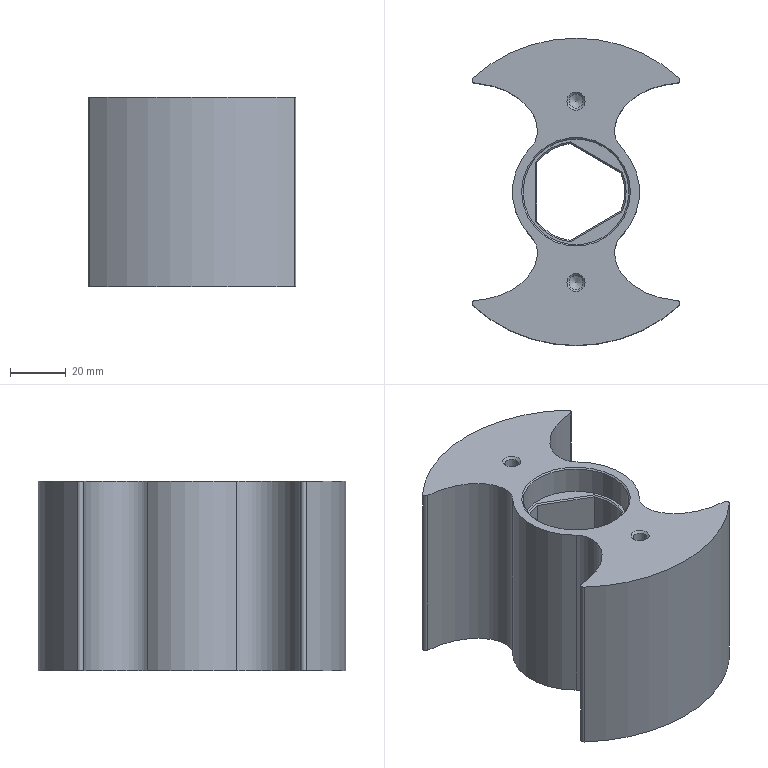NC program | NX | posted with a generic post | part box 74.46 x 110.159 x 68 mm
Lines 1 to 27 of 5030:
N10 G17 G21 G94 G90
(DRILLING_COPY_1 , TOOL : ZXZ)
N12 T01 M6
N14 G54
N16 G17 G0 G90 X-20.25 Y0. S5000 M3
N18 G43 Z30. H1
N20 G94 G81 G98 Z-1. F250. R3.
N22 X20.25
N24 G80
N26 G0 X20.25 Y0. Z30.
N28 M5
(DRILLING_COPY_1_COPY , TOOL : 2.5ZT)
N30 T12 M6
N32 G54
N34 G17 G0 G90 X-20.25 Y0. S2000 M3
N36 G43 Z30. H12
N38 G94 G83 G98 Z-7.751 F120. Q2. R3.
N40 X20.25
N42 G80
N44 G0 X20.25 Y0. Z30.
N46 M5